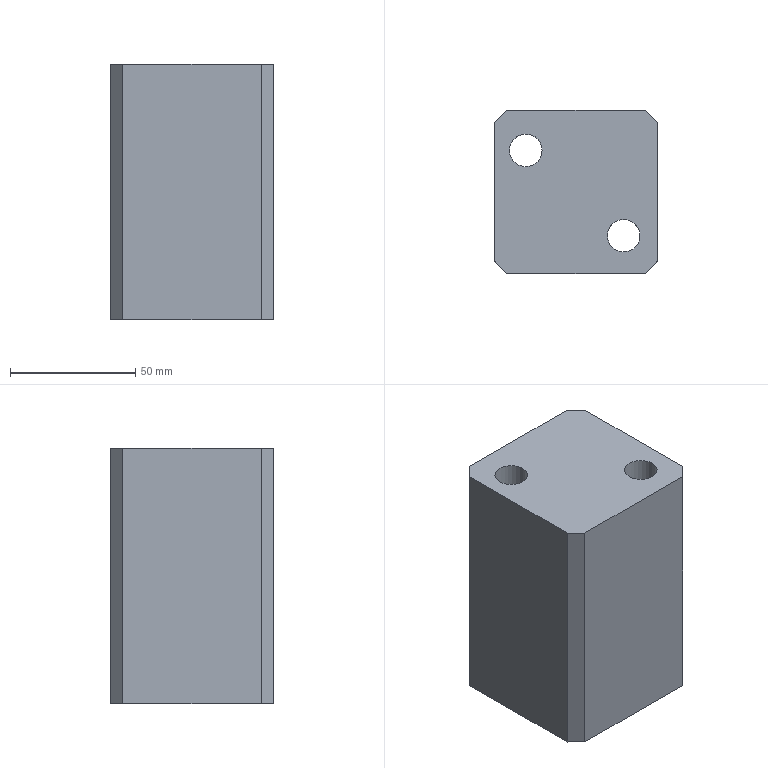Part | STEP file | gslz 2016.10.28-10_id2090_x_t | 1 solid | 20 faces | box 65 x 65 x 102 mm | volume 371101 mm3 | plane 12 | cylinder 6 | cone 2 | commonest cylinder face diameters 10.3 x2 13 x2 20 x2
STEP:
#1=CARTESIAN_POINT('',(0.,0.,0.));
#2=DIRECTION('',(0.,0.,1.));
#3=DIRECTION('',(1.,0.,0.));
#4=AXIS2_PLACEMENT_3D('',#1,#2,#3);
#5=CARTESIAN_POINT('',(-28.5,-279.,3.));
#6=VERTEX_POINT('',#5);
#7=CARTESIAN_POINT('',(-38.5,-279.,3.));
#8=DIRECTION('',(0.,0.,1.));
#9=DIRECTION('',(1.,0.,0.));
#10=AXIS2_PLACEMENT_3D('',#7,#8,#9);
#11=CIRCLE('',#10,10.);
#12=CARTESIAN_POINT('',(-339.5,-320.,3.));
#13=DIRECTION('',(0.,0.,1.));
#14=DIRECTION('',(0.,-1.,0.));
#15=AXIS2_PLACEMENT_3D('',#12,#13,#14);
#16=PLANE('',#15);
#17=CARTESIAN_POINT('',(-41.,301.));
#18=DIRECTION('',(0.,1.));
#19=AXIS2_PLACEMENT_2D('',#17,#18);
#20=CIRCLE('',#19,10.);
#21=(GEOMETRIC_REPRESENTATION_CONTEXT(2)PARAMETRIC_REPRESENTATION_CONTEXT()REPRESENTATION_CONTEXT('',''));
#22=DEFINITIONAL_REPRESENTATION('',(#20),#21);
#23=PCURVE('',#16,#22);
#24=CARTESIAN_POINT('',(-38.5,-279.,42.));
#25=DIRECTION('',(0.,0.,1.));
#26=DIRECTION('',(1.,0.,0.));
#27=AXIS2_PLACEMENT_3D('',#24,#25,#26);
#28=CYLINDRICAL_SURFACE('',#27,10.);
#29=CARTESIAN_POINT('',(0.,-39.));
#30=DIRECTION('',(1.,0.));
#31=VECTOR('',#30,1.);
#32=LINE('',#29,#31);
#33=(GEOMETRIC_REPRESENTATION_CONTEXT(2)PARAMETRIC_REPRESENTATION_CONTEXT()REPRESENTATION_CONTEXT('',''));
#34=DEFINITIONAL_REPRESENTATION('',(#32),#33);
#35=PCURVE('',#28,#34);
#36=SURFACE_CURVE('',#11,(#23,#35),.PCURVE_S1.);
#37=EDGE_CURVE('',#6,#6,#36,.T.);
#38=ORIENTED_EDGE('',*,*,#37,.T.);
#39=EDGE_LOOP('',(#38));
#40=FACE_BOUND('',#39,.T.);
#41=CARTESIAN_POINT('',(-51.,-267.929,3.));
#42=VERTEX_POINT('',#41);
#43=CARTESIAN_POINT('',(-51.,-323.071,3.));
#44=VERTEX_POINT('',#43);
#45=CARTESIAN_POINT('',(-51.,-320.,3.));
#46=DIRECTION('',(0.,-1.,0.));
#47=VECTOR('',#46,1.);
#48=LINE('',#45,#47);
#49=CARTESIAN_POINT('',(0.,288.5));
#50=DIRECTION('',(1.,0.));
#51=VECTOR('',#50,1.);
#52=LINE('',#49,#51);
#53=(GEOMETRIC_REPRESENTATION_CONTEXT(2)PARAMETRIC_REPRESENTATION_CONTEXT()REPRESENTATION_CONTEXT('',''));
#54=DEFINITIONAL_REPRESENTATION('',(#52),#53);
#55=PCURVE('',#16,#54);
#56=CARTESIAN_POINT('',(-51.,612.983,98.));
#57=DIRECTION('',(-1.,0.,0.));
#58=DIRECTION('',(0.,0.,1.));
#59=AXIS2_PLACEMENT_3D('',#56,#57,#58);
#60=PLANE('',#59);
#61=CARTESIAN_POINT('',(-95.,-932.983));
#62=DIRECTION('',(0.,-1.));
#63=VECTOR('',#62,1.);
#64=LINE('',#61,#63);
#65=(GEOMETRIC_REPRESENTATION_CONTEXT(2)PARAMETRIC_REPRESENTATION_CONTEXT()REPRESENTATION_CONTEXT('',''));
#66=DEFINITIONAL_REPRESENTATION('',(#64),#65);
#67=PCURVE('',#60,#66);
#68=SURFACE_CURVE('',#48,(#55,#67),.PCURVE_S1.);
#69=EDGE_CURVE('',#42,#44,#68,.T.);
#70=ORIENTED_EDGE('',*,*,#69,.F.);
#71=CARTESIAN_POINT('',(-46.071,-263.,3.));
#72=VERTEX_POINT('',#71);
#73=CARTESIAN_POINT('',(-47.536,-264.464,3.));
#74=DIRECTION('',(-0.7071,-0.7071,0.));
#75=VECTOR('',#74,1.);
#76=LINE('',#73,#75);
#77=CARTESIAN_POINT('',(-55.536,291.964));
#78=DIRECTION('',(0.7071,-0.7071));
#79=VECTOR('',#78,1.);
#80=LINE('',#77,#79);
#81=(GEOMETRIC_REPRESENTATION_CONTEXT(2)PARAMETRIC_REPRESENTATION_CONTEXT()REPRESENTATION_CONTEXT('',''));
#82=DEFINITIONAL_REPRESENTATION('',(#80),#81);
#83=PCURVE('',#16,#82);
#84=CARTESIAN_POINT('',(-47.536,-264.464,98.));
#85=DIRECTION('',(0.7071,-0.7071,0.));
#86=DIRECTION('',(0.,0.,1.));
#87=AXIS2_PLACEMENT_3D('',#84,#85,#86);
#88=PLANE('',#87);
#89=CARTESIAN_POINT('',(-95.,0.));
#90=DIRECTION('',(0.,1.));
#91=VECTOR('',#90,1.);
#92=LINE('',#89,#91);
#93=(GEOMETRIC_REPRESENTATION_CONTEXT(2)PARAMETRIC_REPRESENTATION_CONTEXT()REPRESENTATION_CONTEXT('',''));
#94=DEFINITIONAL_REPRESENTATION('',(#92),#93);
#95=PCURVE('',#88,#94);
#96=SURFACE_CURVE('',#76,(#83,#95),.PCURVE_S1.);
#97=EDGE_CURVE('',#72,#42,#96,.T.);
#98=ORIENTED_EDGE('',*,*,#97,.F.);
#99=CARTESIAN_POINT('',(9.071,-263.,3.));
#100=VERTEX_POINT('',#99);
#101=CARTESIAN_POINT('',(-339.5,-263.,3.));
#102=DIRECTION('',(-1.,0.,0.));
#103=VECTOR('',#102,1.);
#104=LINE('',#101,#103);
#105=CARTESIAN_POINT('',(-57.,0.));
#106=DIRECTION('',(0.,-1.));
#107=VECTOR('',#106,1.);
#108=LINE('',#105,#107);
#109=(GEOMETRIC_REPRESENTATION_CONTEXT(2)PARAMETRIC_REPRESENTATION_CONTEXT()REPRESENTATION_CONTEXT('',''));
#110=DEFINITIONAL_REPRESENTATION('',(#108),#109);
#111=PCURVE('',#16,#110);
#112=CARTESIAN_POINT('',(-677.884,-263.,98.));
#113=DIRECTION('',(0.,1.,0.));
#114=DIRECTION('',(1.,0.,0.));
#115=AXIS2_PLACEMENT_3D('',#112,#113,#114);
#116=PLANE('',#115);
#117=CARTESIAN_POINT('',(338.384,95.));
#118=DIRECTION('',(-1.,0.));
#119=VECTOR('',#118,1.);
#120=LINE('',#117,#119);
#121=(GEOMETRIC_REPRESENTATION_CONTEXT(2)PARAMETRIC_REPRESENTATION_CONTEXT()REPRESENTATION_CONTEXT('',''));
#122=DEFINITIONAL_REPRESENTATION('',(#120),#121);
#123=PCURVE('',#116,#122);
#124=SURFACE_CURVE('',#104,(#111,#123),.PCURVE_S1.);
#125=EDGE_CURVE('',#100,#72,#124,.T.);
#126=ORIENTED_EDGE('',*,*,#125,.F.);
#127=CARTESIAN_POINT('',(14.,-267.929,3.));
#128=VERTEX_POINT('',#127);
#129=CARTESIAN_POINT('',(12.536,-266.464,3.));
#130=DIRECTION('',(-0.7071,0.7071,0.));
#131=VECTOR('',#130,1.);
#132=LINE('',#129,#131);
#133=CARTESIAN_POINT('',(-53.536,352.036));
#134=DIRECTION('',(-0.7071,-0.7071));
#135=VECTOR('',#134,1.);
#136=LINE('',#133,#135);
#137=(GEOMETRIC_REPRESENTATION_CONTEXT(2)PARAMETRIC_REPRESENTATION_CONTEXT()REPRESENTATION_CONTEXT('',''));
#138=DEFINITIONAL_REPRESENTATION('',(#136),#137);
#139=PCURVE('',#16,#138);
#140=CARTESIAN_POINT('',(12.536,-266.464,98.));
#141=DIRECTION('',(-0.7071,-0.7071,0.));
#142=DIRECTION('',(0.,0.,1.));
#143=AXIS2_PLACEMENT_3D('',#140,#141,#142);
#144=PLANE('',#143);
#145=CARTESIAN_POINT('',(-95.,0.));
#146=DIRECTION('',(0.,1.));
#147=VECTOR('',#146,1.);
#148=LINE('',#145,#147);
#149=(GEOMETRIC_REPRESENTATION_CONTEXT(2)PARAMETRIC_REPRESENTATION_CONTEXT()REPRESENTATION_CONTEXT('',''));
#150=DEFINITIONAL_REPRESENTATION('',(#148),#149);
#151=PCURVE('',#144,#150);
#152=SURFACE_CURVE('',#132,(#139,#151),.PCURVE_S1.);
#153=EDGE_CURVE('',#128,#100,#152,.T.);
#154=ORIENTED_EDGE('',*,*,#153,.F.);
#155=CARTESIAN_POINT('',(14.,-323.071,3.));
#156=VERTEX_POINT('',#155);
#157=CARTESIAN_POINT('',(14.,-320.,3.));
#158=DIRECTION('',(0.,1.,0.));
#159=VECTOR('',#158,1.);
#160=LINE('',#157,#159);
#161=CARTESIAN_POINT('',(0.,353.5));
#162=DIRECTION('',(-1.,0.));
#163=VECTOR('',#162,1.);
#164=LINE('',#161,#163);
#165=(GEOMETRIC_REPRESENTATION_CONTEXT(2)PARAMETRIC_REPRESENTATION_CONTEXT()REPRESENTATION_CONTEXT('',''));
#166=DEFINITIONAL_REPRESENTATION('',(#164),#165);
#167=PCURVE('',#16,#166);
#168=CARTESIAN_POINT('',(14.,612.983,98.));
#169=DIRECTION('',(1.,0.,0.));
#170=DIRECTION('',(0.,0.,-1.));
#171=AXIS2_PLACEMENT_3D('',#168,#169,#170);
#172=PLANE('',#171);
#173=CARTESIAN_POINT('',(95.,-932.983));
#174=DIRECTION('',(0.,1.));
#175=VECTOR('',#174,1.);
#176=LINE('',#173,#175);
#177=(GEOMETRIC_REPRESENTATION_CONTEXT(2)PARAMETRIC_REPRESENTATION_CONTEXT()REPRESENTATION_CONTEXT('',''));
#178=DEFINITIONAL_REPRESENTATION('',(#176),#177);
#179=PCURVE('',#172,#178);
#180=SURFACE_CURVE('',#160,(#167,#179),.PCURVE_S1.);
#181=EDGE_CURVE('',#156,#128,#180,.T.);
#182=ORIENTED_EDGE('',*,*,#181,.F.);
#183=CARTESIAN_POINT('',(9.071,-328.,3.));
#184=VERTEX_POINT('',#183);
#185=CARTESIAN_POINT('',(12.536,-324.536,3.));
#186=DIRECTION('',(0.7071,0.7071,0.));
#187=VECTOR('',#186,1.);
#188=LINE('',#185,#187);
#189=CARTESIAN_POINT('',(4.536,352.036));
#190=DIRECTION('',(-0.7071,0.7071));
#191=VECTOR('',#190,1.);
#192=LINE('',#189,#191);
#193=(GEOMETRIC_REPRESENTATION_CONTEXT(2)PARAMETRIC_REPRESENTATION_CONTEXT()REPRESENTATION_CONTEXT('',''));
#194=DEFINITIONAL_REPRESENTATION('',(#192),#193);
#195=PCURVE('',#16,#194);
#196=CARTESIAN_POINT('',(12.536,-324.536,98.));
#197=DIRECTION('',(-0.7071,0.7071,0.));
#198=DIRECTION('',(0.,0.,-1.));
#199=AXIS2_PLACEMENT_3D('',#196,#197,#198);
#200=PLANE('',#199);
#201=CARTESIAN_POINT('',(95.,0.));
#202=DIRECTION('',(0.,-1.));
#203=VECTOR('',#202,1.);
#204=LINE('',#201,#203);
#205=(GEOMETRIC_REPRESENTATION_CONTEXT(2)PARAMETRIC_REPRESENTATION_CONTEXT()REPRESENTATION_CONTEXT('',''));
#206=DEFINITIONAL_REPRESENTATION('',(#204),#205);
#207=PCURVE('',#200,#206);
#208=SURFACE_CURVE('',#188,(#195,#207),.PCURVE_S1.);
#209=EDGE_CURVE('',#184,#156,#208,.T.);
#210=ORIENTED_EDGE('',*,*,#209,.F.);
#211=CARTESIAN_POINT('',(-46.071,-328.,3.));
#212=VERTEX_POINT('',#211);
#213=CARTESIAN_POINT('',(-339.5,-328.,3.));
#214=DIRECTION('',(1.,0.,0.));
#215=VECTOR('',#214,1.);
#216=LINE('',#213,#215);
#217=CARTESIAN_POINT('',(8.,0.));
#218=DIRECTION('',(0.,1.));
#219=VECTOR('',#218,1.);
#220=LINE('',#217,#219);
#221=(GEOMETRIC_REPRESENTATION_CONTEXT(2)PARAMETRIC_REPRESENTATION_CONTEXT()REPRESENTATION_CONTEXT('',''));
#222=DEFINITIONAL_REPRESENTATION('',(#220),#221);
#223=PCURVE('',#16,#222);
#224=CARTESIAN_POINT('',(-677.035,-328.,98.));
#225=DIRECTION('',(0.,-1.,0.));
#226=DIRECTION('',(-1.,0.,0.));
#227=AXIS2_PLACEMENT_3D('',#224,#225,#226);
#228=PLANE('',#227);
#229=CARTESIAN_POINT('',(-337.535,95.));
#230=DIRECTION('',(-1.,0.));
#231=VECTOR('',#230,1.);
#232=LINE('',#229,#231);
#233=(GEOMETRIC_REPRESENTATION_CONTEXT(2)PARAMETRIC_REPRESENTATION_CONTEXT()REPRESENTATION_CONTEXT('',''));
#234=DEFINITIONAL_REPRESENTATION('',(#232),#233);
#235=PCURVE('',#228,#234);
#236=SURFACE_CURVE('',#216,(#223,#235),.PCURVE_S1.);
#237=EDGE_CURVE('',#212,#184,#236,.T.);
#238=ORIENTED_EDGE('',*,*,#237,.F.);
#239=CARTESIAN_POINT('',(-47.536,-326.536,3.));
#240=DIRECTION('',(0.7071,-0.7071,0.));
#241=VECTOR('',#240,1.);
#242=LINE('',#239,#241);
#243=CARTESIAN_POINT('',(6.536,291.964));
#244=DIRECTION('',(0.7071,0.7071));
#245=VECTOR('',#244,1.);
#246=LINE('',#243,#245);
#247=(GEOMETRIC_REPRESENTATION_CONTEXT(2)PARAMETRIC_REPRESENTATION_CONTEXT()REPRESENTATION_CONTEXT('',''));
#248=DEFINITIONAL_REPRESENTATION('',(#246),#247);
#249=PCURVE('',#16,#248);
#250=CARTESIAN_POINT('',(-47.536,-326.536,98.));
#251=DIRECTION('',(0.7071,0.7071,0.));
#252=DIRECTION('',(0.,0.,-1.));
#253=AXIS2_PLACEMENT_3D('',#250,#251,#252);
#254=PLANE('',#253);
#255=CARTESIAN_POINT('',(95.,0.));
#256=DIRECTION('',(0.,-1.));
#257=VECTOR('',#256,1.);
#258=LINE('',#255,#257);
#259=(GEOMETRIC_REPRESENTATION_CONTEXT(2)PARAMETRIC_REPRESENTATION_CONTEXT()REPRESENTATION_CONTEXT('',''));
#260=DEFINITIONAL_REPRESENTATION('',(#258),#259);
#261=PCURVE('',#254,#260);
#262=SURFACE_CURVE('',#242,(#249,#261),.PCURVE_S1.);
#263=EDGE_CURVE('',#44,#212,#262,.T.);
#264=ORIENTED_EDGE('',*,*,#263,.F.);
#265=EDGE_LOOP('',(#70,#98,#126,#154,#182,#210,#238,#264));
#266=FACE_BOUND('',#265,.T.);
#267=CARTESIAN_POINT('',(10.5,-313.,3.));
#268=VERTEX_POINT('',#267);
#269=CARTESIAN_POINT('',(0.5,-313.,3.));
#270=DIRECTION('',(0.,0.,1.));
#271=DIRECTION('',(1.,0.,0.));
#272=AXIS2_PLACEMENT_3D('',#269,#270,#271);
#273=CIRCLE('',#272,10.);
#274=CARTESIAN_POINT('',(-7.,340.));
#275=DIRECTION('',(0.,1.));
#276=AXIS2_PLACEMENT_2D('',#274,#275);
#277=CIRCLE('',#276,10.);
#278=(GEOMETRIC_REPRESENTATION_CONTEXT(2)PARAMETRIC_REPRESENTATION_CONTEXT()REPRESENTATION_CONTEXT('',''));
#279=DEFINITIONAL_REPRESENTATION('',(#277),#278);
#280=PCURVE('',#16,#279);
#281=CARTESIAN_POINT('',(0.5,-313.,42.));
#282=DIRECTION('',(0.,0.,1.));
#283=DIRECTION('',(1.,0.,0.));
#284=AXIS2_PLACEMENT_3D('',#281,#282,#283);
#285=CYLINDRICAL_SURFACE('',#284,10.);
#286=CARTESIAN_POINT('',(0.,-39.));
#287=DIRECTION('',(1.,0.));
#288=VECTOR('',#287,1.);
#289=LINE('',#286,#288);
#290=(GEOMETRIC_REPRESENTATION_CONTEXT(2)PARAMETRIC_REPRESENTATION_CONTEXT()REPRESENTATION_CONTEXT('',''));
#291=DEFINITIONAL_REPRESENTATION('',(#289),#290);
#292=PCURVE('',#285,#291);
#293=SURFACE_CURVE('',#273,(#280,#292),.PCURVE_S1.);
#294=EDGE_CURVE('',#268,#268,#293,.T.);
#295=ORIENTED_EDGE('',*,*,#294,.T.);
#296=EDGE_LOOP('',(#295));
#297=FACE_BOUND('',#296,.T.);
#298=CARTESIAN_POINT('',(-33.35,-314.,3.));
#299=VERTEX_POINT('',#298);
#300=CARTESIAN_POINT('',(-38.5,-314.,3.));
#301=DIRECTION('',(0.,0.,-1.));
#302=DIRECTION('',(1.,0.,0.));
#303=AXIS2_PLACEMENT_3D('',#300,#301,#302);
#304=CIRCLE('',#303,5.15);
#305=CARTESIAN_POINT('',(-6.,306.15));
#306=CARTESIAN_POINT('',(2.92,306.15));
#307=CARTESIAN_POINT('',(-1.54,298.425));
#308=CARTESIAN_POINT('',(-6.,290.7));
#309=CARTESIAN_POINT('',(-10.46,298.425));
#310=CARTESIAN_POINT('',(-14.92,306.15));
#311=CARTESIAN_POINT('',(-6.,306.15));
#312=(BOUNDED_CURVE()B_SPLINE_CURVE(2,(#305,#306,#307,#308,#309,#310,#311),.UNSPECIFIED.,.T.,.F.)B_SPLINE_CURVE_WITH_KNOTS((1,2,2,2,2,1),(-2.094,0.,2.094,4.189,6.283,8.378),.UNSPECIFIED.)CURVE()GEOMETRIC_REPRESENTATION_ITEM()RATIONAL_B_SPLINE_CURVE((1.,0.5,1.,0.5,1.,0.5,1.))REPRESENTATION_ITEM(''));
#313=(GEOMETRIC_REPRESENTATION_CONTEXT(2)PARAMETRIC_REPRESENTATION_CONTEXT()REPRESENTATION_CONTEXT('',''));
#314=DEFINITIONAL_REPRESENTATION('',(#312),#313);
#315=PCURVE('',#16,#314);
#316=CARTESIAN_POINT('',(-38.5,-314.,-12.));
#317=DIRECTION('',(0.,0.,1.));
#318=DIRECTION('',(-1.,0.,0.));
#319=AXIS2_PLACEMENT_3D('',#316,#317,#318);
#320=CYLINDRICAL_SURFACE('',#319,5.15);
#321=CARTESIAN_POINT('',(9.425,15.));
#322=DIRECTION('',(-1.,0.));
#323=VECTOR('',#322,1.);
#324=LINE('',#321,#323);
#325=(GEOMETRIC_REPRESENTATION_CONTEXT(2)PARAMETRIC_REPRESENTATION_CONTEXT()REPRESENTATION_CONTEXT('',''));
#326=DEFINITIONAL_REPRESENTATION('',(#324),#325);
#327=PCURVE('',#320,#326);
#328=SURFACE_CURVE('',#304,(#315,#327),.PCURVE_S1.);
#329=EDGE_CURVE('',#299,#299,#328,.T.);
#330=ORIENTED_EDGE('',*,*,#329,.F.);
#331=EDGE_LOOP('',(#330));
#332=FACE_BOUND('',#331,.T.);
#333=CARTESIAN_POINT('',(5.65,-279.,3.));
#334=VERTEX_POINT('',#333);
#335=CARTESIAN_POINT('',(0.5,-279.,3.));
#336=DIRECTION('',(0.,0.,1.));
#337=DIRECTION('',(1.,0.,0.));
#338=AXIS2_PLACEMENT_3D('',#335,#336,#337);
#339=CIRCLE('',#338,5.15);
#340=CARTESIAN_POINT('',(-41.,340.));
#341=DIRECTION('',(0.,1.));
#342=AXIS2_PLACEMENT_2D('',#340,#341);
#343=CIRCLE('',#342,5.15);
#344=(GEOMETRIC_REPRESENTATION_CONTEXT(2)PARAMETRIC_REPRESENTATION_CONTEXT()REPRESENTATION_CONTEXT('',''));
#345=DEFINITIONAL_REPRESENTATION('',(#343),#344);
#346=PCURVE('',#16,#345);
#347=CARTESIAN_POINT('',(0.5,-279.,-12.));
#348=DIRECTION('',(0.,0.,1.));
#349=DIRECTION('',(-1.,0.,0.));
#350=AXIS2_PLACEMENT_3D('',#347,#348,#349);
#351=CYLINDRICAL_SURFACE('',#350,5.15);
#352=CARTESIAN_POINT('',(3.142,15.));
#353=DIRECTION('',(1.,0.));
#354=VECTOR('',#353,1.);
#355=LINE('',#352,#354);
#356=(GEOMETRIC_REPRESENTATION_CONTEXT(2)PARAMETRIC_REPRESENTATION_CONTEXT()REPRESENTATION_CONTEXT('',''));
#357=DEFINITIONAL_REPRESENTATION('',(#355),#356);
#358=PCURVE('',#351,#357);
#359=SURFACE_CURVE('',#339,(#346,#358),.PCURVE_S1.);
#360=EDGE_CURVE('',#334,#334,#359,.T.);
#361=ORIENTED_EDGE('',*,*,#360,.T.);
#362=EDGE_LOOP('',(#361));
#363=FACE_BOUND('',#362,.T.);
#364=ADVANCED_FACE('',(#40,#266,#297,#332,#363),#16,.F.);
#365=CARTESIAN_POINT('',(-33.35,-314.,23.));
#366=VERTEX_POINT('',#365);
#367=CARTESIAN_POINT('',(-38.5,-314.,23.));
#368=DIRECTION('',(0.,0.,1.));
#369=DIRECTION('',(1.,0.,0.));
#370=AXIS2_PLACEMENT_3D('',#367,#368,#369);
#371=CIRCLE('',#370,5.15);
#372=CARTESIAN_POINT('',(3.142,35.));
#373=DIRECTION('',(1.,0.));
#374=VECTOR('',#373,1.);
#375=LINE('',#372,#374);
#376=(GEOMETRIC_REPRESENTATION_CONTEXT(2)PARAMETRIC_REPRESENTATION_CONTEXT()REPRESENTATION_CONTEXT('',''));
#377=DEFINITIONAL_REPRESENTATION('',(#375),#376);
#378=PCURVE('',#320,#377);
#379=CARTESIAN_POINT('',(-38.5,-314.,23.));
#380=DIRECTION('',(0.,0.,-1.));
#381=DIRECTION('',(1.,0.,0.));
#382=AXIS2_PLACEMENT_3D('',#379,#380,#381);
#383=CONICAL_SURFACE('',#382,5.15,1.03);
#384=CARTESIAN_POINT('',(6.283,0.));
#385=DIRECTION('',(-1.,0.));
#386=VECTOR('',#385,1.);
#387=LINE('',#384,#386);
#388=(GEOMETRIC_REPRESENTATION_CONTEXT(2)PARAMETRIC_REPRESENTATION_CONTEXT()REPRESENTATION_CONTEXT('',''));
#389=DEFINITIONAL_REPRESENTATION('',(#387),#388);
#390=PCURVE('',#383,#389);
#391=SURFACE_CURVE('',#371,(#378,#390),.PCURVE_S1.);
#392=EDGE_CURVE('',#366,#366,#391,.T.);
#393=ORIENTED_EDGE('',*,*,#392,.F.);
#394=CARTESIAN_POINT('',(-33.35,-314.,3.));
#395=CARTESIAN_POINT('',(-33.35,-314.,23.));
#396=B_SPLINE_CURVE_WITH_KNOTS('',1,(#394,#395),.UNSPECIFIED.,.F.,.F.,(2,2),(15.,35.),.PIECEWISE_BEZIER_KNOTS.);
#397=CARTESIAN_POINT('',(3.142,0.));
#398=DIRECTION('',(0.,1.));
#399=VECTOR('',#398,1.);
#400=LINE('',#397,#399);
#401=(GEOMETRIC_REPRESENTATION_CONTEXT(2)PARAMETRIC_REPRESENTATION_CONTEXT()REPRESENTATION_CONTEXT('',''));
#402=DEFINITIONAL_REPRESENTATION('',(#400),#401);
#403=PCURVE('',#320,#402);
#404=CARTESIAN_POINT('',(9.425,0.));
#405=DIRECTION('',(0.,1.));
#406=VECTOR('',#405,1.);
#407=LINE('',#404,#406);
#408=(GEOMETRIC_REPRESENTATION_CONTEXT(2)PARAMETRIC_REPRESENTATION_CONTEXT()REPRESENTATION_CONTEXT('',''));
#409=DEFINITIONAL_REPRESENTATION('',(#407),#408);
#410=PCURVE('',#320,#409);
#411=SEAM_CURVE('',#396,(#403,#410),.PCURVE_S1.);
#412=EDGE_CURVE('',#299,#366,#411,.T.);
#413=ORIENTED_EDGE('',*,*,#412,.F.);
#414=ORIENTED_EDGE('',*,*,#329,.F.);
#415=ORIENTED_EDGE('',*,*,#412,.T.);
#416=EDGE_LOOP('',(#393,#413,#414,#415));
#417=FACE_BOUND('',#416,.F.);
#418=ADVANCED_FACE('',(#417),#320,.F.);
#419=CARTESIAN_POINT('',(7.,-313.,70.));
#420=VERTEX_POINT('',#419);
#421=CARTESIAN_POINT('',(0.5,-313.,70.));
#422=DIRECTION('',(0.,0.,1.));
#423=DIRECTION('',(1.,0.,0.));
#424=AXIS2_PLACEMENT_3D('',#421,#422,#423);
#425=CIRCLE('',#424,6.5);
#426=CARTESIAN_POINT('',(0.5,-313.,70.));
#427=DIRECTION('',(0.,0.,1.));
#428=DIRECTION('',(1.,0.,0.));
#429=AXIS2_PLACEMENT_3D('',#426,#427,#428);
#430=PLANE('',#429);
#431=CARTESIAN_POINT('',(0.,0.));
#432=DIRECTION('',(1.,0.));
#433=AXIS2_PLACEMENT_2D('',#431,#432);
#434=CIRCLE('',#433,6.5);
#435=(GEOMETRIC_REPRESENTATION_CONTEXT(2)PARAMETRIC_REPRESENTATION_CONTEXT()REPRESENTATION_CONTEXT('',''));
#436=DEFINITIONAL_REPRESENTATION('',(#434),#435);
#437=PCURVE('',#430,#436);
#438=CARTESIAN_POINT('',(0.5,-313.,87.));
#439=DIRECTION('',(0.,0.,1.));
#440=DIRECTION('',(1.,0.,0.));
#441=AXIS2_PLACEMENT_3D('',#438,#439,#440);
#442=CYLINDRICAL_SURFACE('',#441,6.5);
#443=CARTESIAN_POINT('',(0.,-17.));
#444=DIRECTION('',(1.,0.));
#445=VECTOR('',#444,1.);
#446=LINE('',#443,#445);
#447=(GEOMETRIC_REPRESENTATION_CONTEXT(2)PARAMETRIC_REPRESENTATION_CONTEXT()REPRESENTATION_CONTEXT('',''));
#448=DEFINITIONAL_REPRESENTATION('',(#446),#447);
#449=PCURVE('',#442,#448);
#450=SURFACE_CURVE('',#425,(#437,#449),.PCURVE_S1.);
#451=EDGE_CURVE('',#420,#420,#450,.T.);
#452=ORIENTED_EDGE('',*,*,#451,.T.);
#453=EDGE_LOOP('',(#452));
#454=FACE_BOUND('',#453,.T.);
#455=CARTESIAN_POINT('',(10.5,-313.,70.));
#456=VERTEX_POINT('',#455);
#457=CARTESIAN_POINT('',(0.5,-313.,70.));
#458=DIRECTION('',(0.,0.,1.));
#459=DIRECTION('',(1.,0.,0.));
#460=AXIS2_PLACEMENT_3D('',#457,#458,#459);
#461=CIRCLE('',#460,10.);
#462=CARTESIAN_POINT('',(0.,0.));
#463=DIRECTION('',(1.,0.));
#464=AXIS2_PLACEMENT_2D('',#462,#463);
#465=CIRCLE('',#464,10.);
#466=(GEOMETRIC_REPRESENTATION_CONTEXT(2)PARAMETRIC_REPRESENTATION_CONTEXT()REPRESENTATION_CONTEXT('',''));
#467=DEFINITIONAL_REPRESENTATION('',(#465),#466);
#468=PCURVE('',#430,#467);
#469=CARTESIAN_POINT('',(0.,28.));
#470=DIRECTION('',(1.,0.));
#471=VECTOR('',#470,1.);
#472=LINE('',#469,#471);
#473=(GEOMETRIC_REPRESENTATION_CONTEXT(2)PARAMETRIC_REPRESENTATION_CONTEXT()REPRESENTATION_CONTEXT('',''));
#474=DEFINITIONAL_REPRESENTATION('',(#472),#473);
#475=PCURVE('',#285,#474);
#476=SURFACE_CURVE('',#461,(#468,#475),.PCURVE_S1.);
#477=EDGE_CURVE('',#456,#456,#476,.T.);
#478=ORIENTED_EDGE('',*,*,#477,.F.);
#479=EDGE_LOOP('',(#478));
#480=FACE_BOUND('',#479,.T.);
#481=ADVANCED_FACE('',(#454,#480),#430,.F.);
#482=CARTESIAN_POINT('',(-32.,-279.,70.));
#483=VERTEX_POINT('',#482);
#484=CARTESIAN_POINT('',(-38.5,-279.,70.));
#485=DIRECTION('',(0.,0.,1.));
#486=DIRECTION('',(1.,0.,0.));
#487=AXIS2_PLACEMENT_3D('',#484,#485,#486);
#488=CIRCLE('',#487,6.5);
#489=CARTESIAN_POINT('',(-38.5,-279.,70.));
#490=DIRECTION('',(0.,0.,1.));
#491=DIRECTION('',(1.,0.,0.));
#492=AXIS2_PLACEMENT_3D('',#489,#490,#491);
#493=PLANE('',#492);
#494=CARTESIAN_POINT('',(0.,0.));
#495=DIRECTION('',(1.,0.));
#496=AXIS2_PLACEMENT_2D('',#494,#495);
#497=CIRCLE('',#496,6.5);
#498=(GEOMETRIC_REPRESENTATION_CONTEXT(2)PARAMETRIC_REPRESENTATION_CONTEXT()REPRESENTATION_CONTEXT('',''));
#499=DEFINITIONAL_REPRESENTATION('',(#497),#498);
#500=PCURVE('',#493,#499);
#501=CARTESIAN_POINT('',(-38.5,-279.,87.));
#502=DIRECTION('',(0.,0.,1.));
#503=DIRECTION('',(1.,0.,0.));
#504=AXIS2_PLACEMENT_3D('',#501,#502,#503);
#505=CYLINDRICAL_SURFACE('',#504,6.5);
#506=CARTESIAN_POINT('',(0.,-17.));
#507=DIRECTION('',(1.,0.));
#508=VECTOR('',#507,1.);
#509=LINE('',#506,#508);
#510=(GEOMETRIC_REPRESENTATION_CONTEXT(2)PARAMETRIC_REPRESENTATION_CONTEXT()REPRESENTATION_CONTEXT('',''));
#511=DEFINITIONAL_REPRESENTATION('',(#509),#510);
#512=PCURVE('',#505,#511);
#513=SURFACE_CURVE('',#488,(#500,#512),.PCURVE_S1.);
#514=EDGE_CURVE('',#483,#483,#513,.T.);
#515=ORIENTED_EDGE('',*,*,#514,.T.);
#516=EDGE_LOOP('',(#515));
#517=FACE_BOUND('',#516,.T.);
#518=CARTESIAN_POINT('',(-28.5,-279.,70.));
#519=VERTEX_POINT('',#518);
#520=CARTESIAN_POINT('',(-38.5,-279.,70.));
#521=DIRECTION('',(0.,0.,1.));
#522=DIRECTION('',(1.,0.,0.));
#523=AXIS2_PLACEMENT_3D('',#520,#521,#522);
#524=CIRCLE('',#523,10.);
#525=CARTESIAN_POINT('',(0.,0.));
#526=DIRECTION('',(1.,0.));
#527=AXIS2_PLACEMENT_2D('',#525,#526);
#528=CIRCLE('',#527,10.);
#529=(GEOMETRIC_REPRESENTATION_CONTEXT(2)PARAMETRIC_REPRESENTATION_CONTEXT()REPRESENTATION_CONTEXT('',''));
#530=DEFINITIONAL_REPRESENTATION('',(#528),#529);
#531=PCURVE('',#493,#530);
#532=CARTESIAN_POINT('',(0.,28.));
#533=DIRECTION('',(1.,0.));
#534=VECTOR('',#533,1.);
#535=LINE('',#532,#534);
#536=(GEOMETRIC_REPRESENTATION_CONTEXT(2)PARAMETRIC_REPRESENTATION_CONTEXT()REPRESENTATION_CONTEXT('',''));
#537=DEFINITIONAL_REPRESENTATION('',(#535),#536);
#538=PCURVE('',#28,#537);
#539=SURFACE_CURVE('',#524,(#531,#538),.PCURVE_S1.);
#540=EDGE_CURVE('',#519,#519,#539,.T.);
#541=ORIENTED_EDGE('',*,*,#540,.F.);
#542=EDGE_LOOP('',(#541));
#543=FACE_BOUND('',#542,.T.);
#544=ADVANCED_FACE('',(#517,#543),#493,.F.);
#545=ORIENTED_EDGE('',*,*,#294,.T.);
#546=CARTESIAN_POINT('',(10.5,-313.,3.));
#547=CARTESIAN_POINT('',(10.5,-313.,70.));
#548=B_SPLINE_CURVE_WITH_KNOTS('',1,(#546,#547),.UNSPECIFIED.,.F.,.F.,(2,2),(-39.,28.),.PIECEWISE_BEZIER_KNOTS.);
#549=CARTESIAN_POINT('',(6.283,0.));
#550=DIRECTION('',(0.,1.));
#551=VECTOR('',#550,1.);
#552=LINE('',#549,#551);
#553=(GEOMETRIC_REPRESENTATION_CONTEXT(2)PARAMETRIC_REPRESENTATION_CONTEXT()REPRESENTATION_CONTEXT('',''));
#554=DEFINITIONAL_REPRESENTATION('',(#552),#553);
#555=PCURVE('',#285,#554);
#556=CARTESIAN_POINT('',(0.,0.));
#557=DIRECTION('',(0.,1.));
#558=VECTOR('',#557,1.);
#559=LINE('',#556,#558);
#560=(GEOMETRIC_REPRESENTATION_CONTEXT(2)PARAMETRIC_REPRESENTATION_CONTEXT()REPRESENTATION_CONTEXT('',''));
#561=DEFINITIONAL_REPRESENTATION('',(#559),#560);
#562=PCURVE('',#285,#561);
#563=SEAM_CURVE('',#548,(#555,#562),.PCURVE_S1.);
#564=EDGE_CURVE('',#268,#456,#563,.T.);
#565=ORIENTED_EDGE('',*,*,#564,.T.);
#566=ORIENTED_EDGE('',*,*,#477,.F.);
#567=ORIENTED_EDGE('',*,*,#564,.F.);
#568=EDGE_LOOP('',(#545,#565,#566,#567));
#569=FACE_BOUND('',#568,.F.);
#570=ADVANCED_FACE('',(#569),#285,.F.);
#571=ORIENTED_EDGE('',*,*,#237,.T.);
#572=CARTESIAN_POINT('',(9.071,-328.,105.));
#573=VERTEX_POINT('',#572);
#574=CARTESIAN_POINT('',(9.071,-328.,98.));
#575=DIRECTION('',(0.,0.,-1.));
#576=VECTOR('',#575,1.);
#577=LINE('',#574,#576);
#578=CARTESIAN_POINT('',(-686.106,0.));
#579=DIRECTION('',(0.,1.));
#580=VECTOR('',#579,1.);
#581=LINE('',#578,#580);
#582=(GEOMETRIC_REPRESENTATION_CONTEXT(2)PARAMETRIC_REPRESENTATION_CONTEXT()REPRESENTATION_CONTEXT('',''));
#583=DEFINITIONAL_REPRESENTATION('',(#581),#582);
#584=PCURVE('',#228,#583);
#585=CARTESIAN_POINT('',(0.,4.899));
#586=DIRECTION('',(1.,0.));
#587=VECTOR('',#586,1.);
#588=LINE('',#585,#587);
#589=(GEOMETRIC_REPRESENTATION_CONTEXT(2)PARAMETRIC_REPRESENTATION_CONTEXT()REPRESENTATION_CONTEXT('',''));
#590=DEFINITIONAL_REPRESENTATION('',(#588),#589);
#591=PCURVE('',#200,#590);
#592=SURFACE_CURVE('',#577,(#584,#591),.PCURVE_S1.);
#593=EDGE_CURVE('',#573,#184,#592,.T.);
#594=ORIENTED_EDGE('',*,*,#593,.F.);
#595=CARTESIAN_POINT('',(-46.071,-328.,105.));
#596=VERTEX_POINT('',#595);
#597=CARTESIAN_POINT('',(46.5,-328.,105.));
#598=DIRECTION('',(1.,0.,0.));
#599=VECTOR('',#598,1.);
#600=LINE('',#597,#599);
#601=CARTESIAN_POINT('',(-723.535,-7.));
#602=DIRECTION('',(-1.,0.));
#603=VECTOR('',#602,1.);
#604=LINE('',#601,#603);
#605=(GEOMETRIC_REPRESENTATION_CONTEXT(2)PARAMETRIC_REPRESENTATION_CONTEXT()REPRESENTATION_CONTEXT('',''));
#606=DEFINITIONAL_REPRESENTATION('',(#604),#605);
#607=PCURVE('',#228,#606);
#608=CARTESIAN_POINT('',(46.5,87.,105.));
#609=DIRECTION('',(0.,0.,1.));
#610=DIRECTION('',(-1.,0.,0.));
#611=AXIS2_PLACEMENT_3D('',#608,#609,#610);
#612=PLANE('',#611);
#613=CARTESIAN_POINT('',(0.,415.));
#614=DIRECTION('',(-1.,0.));
#615=VECTOR('',#614,1.);
#616=LINE('',#613,#615);
#617=(GEOMETRIC_REPRESENTATION_CONTEXT(2)PARAMETRIC_REPRESENTATION_CONTEXT()REPRESENTATION_CONTEXT('',''));
#618=DEFINITIONAL_REPRESENTATION('',(#616),#617);
#619=PCURVE('',#612,#618);
#620=SURFACE_CURVE('',#600,(#607,#619),.PCURVE_S1.);
#621=EDGE_CURVE('',#596,#573,#620,.T.);
#622=ORIENTED_EDGE('',*,*,#621,.F.);
#623=CARTESIAN_POINT('',(-46.071,-328.,98.));
#624=DIRECTION('',(0.,0.,1.));
#625=VECTOR('',#624,1.);
#626=LINE('',#623,#625);
#627=CARTESIAN_POINT('',(-630.964,0.));
#628=DIRECTION('',(0.,-1.));
#629=VECTOR('',#628,1.);
#630=LINE('',#627,#629);
#631=(GEOMETRIC_REPRESENTATION_CONTEXT(2)PARAMETRIC_REPRESENTATION_CONTEXT()REPRESENTATION_CONTEXT('',''));
#632=DEFINITIONAL_REPRESENTATION('',(#630),#631);
#633=PCURVE('',#228,#632);
#634=CARTESIAN_POINT('',(0.,-2.071));
#635=DIRECTION('',(-1.,0.));
#636=VECTOR('',#635,1.);
#637=LINE('',#634,#636);
#638=(GEOMETRIC_REPRESENTATION_CONTEXT(2)PARAMETRIC_REPRESENTATION_CONTEXT()REPRESENTATION_CONTEXT('',''));
#639=DEFINITIONAL_REPRESENTATION('',(#637),#638);
#640=PCURVE('',#254,#639);
#641=SURFACE_CURVE('',#626,(#633,#640),.PCURVE_S1.);
#642=EDGE_CURVE('',#212,#596,#641,.T.);
#643=ORIENTED_EDGE('',*,*,#642,.F.);
#644=EDGE_LOOP('',(#571,#594,#622,#643));
#645=FACE_BOUND('',#644,.T.);
#646=ADVANCED_FACE('',(#645),#228,.T.);
#647=CARTESIAN_POINT('',(-51.,-267.929,105.));
#648=VERTEX_POINT('',#647);
#649=CARTESIAN_POINT('',(-51.,-323.071,105.));
#650=VERTEX_POINT('',#649);
#651=CARTESIAN_POINT('',(-51.,87.,105.));
#652=DIRECTION('',(0.,-1.,0.));
#653=VECTOR('',#652,1.);
#654=LINE('',#651,#653);
#655=CARTESIAN_POINT('',(7.,-525.983));
#656=DIRECTION('',(0.,-1.));
#657=VECTOR('',#656,1.);
#658=LINE('',#655,#657);
#659=(GEOMETRIC_REPRESENTATION_CONTEXT(2)PARAMETRIC_REPRESENTATION_CONTEXT()REPRESENTATION_CONTEXT('',''));
#660=DEFINITIONAL_REPRESENTATION('',(#658),#659);
#661=PCURVE('',#60,#660);
#662=CARTESIAN_POINT('',(97.5,0.));
#663=DIRECTION('',(0.,1.));
#664=VECTOR('',#663,1.);
#665=LINE('',#662,#664);
#666=(GEOMETRIC_REPRESENTATION_CONTEXT(2)PARAMETRIC_REPRESENTATION_CONTEXT()REPRESENTATION_CONTEXT('',''));
#667=DEFINITIONAL_REPRESENTATION('',(#665),#666);
#668=PCURVE('',#612,#667);
#669=SURFACE_CURVE('',#654,(#661,#668),.PCURVE_S1.);
#670=EDGE_CURVE('',#648,#650,#669,.T.);
#671=ORIENTED_EDGE('',*,*,#670,.F.);
#672=CARTESIAN_POINT('',(-51.,-267.929,98.));
#673=DIRECTION('',(0.,0.,1.));
#674=VECTOR('',#673,1.);
#675=LINE('',#672,#674);
#676=CARTESIAN_POINT('',(0.,-880.911));
#677=DIRECTION('',(1.,0.));
#678=VECTOR('',#677,1.);
#679=LINE('',#676,#678);
#680=(GEOMETRIC_REPRESENTATION_CONTEXT(2)PARAMETRIC_REPRESENTATION_CONTEXT()REPRESENTATION_CONTEXT('',''));
#681=DEFINITIONAL_REPRESENTATION('',(#679),#680);
#682=PCURVE('',#60,#681);
#683=CARTESIAN_POINT('',(0.,4.899));
#684=DIRECTION('',(1.,0.));
#685=VECTOR('',#684,1.);
#686=LINE('',#683,#685);
#687=(GEOMETRIC_REPRESENTATION_CONTEXT(2)PARAMETRIC_REPRESENTATION_CONTEXT()REPRESENTATION_CONTEXT('',''));
#688=DEFINITIONAL_REPRESENTATION('',(#686),#687);
#689=PCURVE('',#88,#688);
#690=SURFACE_CURVE('',#675,(#682,#689),.PCURVE_S1.);
#691=EDGE_CURVE('',#42,#648,#690,.T.);
#692=ORIENTED_EDGE('',*,*,#691,.F.);
#693=ORIENTED_EDGE('',*,*,#69,.T.);
#694=CARTESIAN_POINT('',(-51.,-323.071,98.));
#695=DIRECTION('',(0.,0.,-1.));
#696=VECTOR('',#695,1.);
#697=LINE('',#694,#696);
#698=CARTESIAN_POINT('',(0.,-936.054));
#699=DIRECTION('',(-1.,0.));
#700=VECTOR('',#699,1.);
#701=LINE('',#698,#700);
#702=(GEOMETRIC_REPRESENTATION_CONTEXT(2)PARAMETRIC_REPRESENTATION_CONTEXT()REPRESENTATION_CONTEXT('',''));
#703=DEFINITIONAL_REPRESENTATION('',(#701),#702);
#704=PCURVE('',#60,#703);
#705=CARTESIAN_POINT('',(0.,4.899));
#706=DIRECTION('',(1.,0.));
#707=VECTOR('',#706,1.);
#708=LINE('',#705,#707);
#709=(GEOMETRIC_REPRESENTATION_CONTEXT(2)PARAMETRIC_REPRESENTATION_CONTEXT()REPRESENTATION_CONTEXT('',''));
#710=DEFINITIONAL_REPRESENTATION('',(#708),#709);
#711=PCURVE('',#254,#710);
#712=SURFACE_CURVE('',#697,(#704,#711),.PCURVE_S1.);
#713=EDGE_CURVE('',#650,#44,#712,.T.);
#714=ORIENTED_EDGE('',*,*,#713,.F.);
#715=EDGE_LOOP('',(#671,#692,#693,#714));
#716=FACE_BOUND('',#715,.T.);
#717=ADVANCED_FACE('',(#716),#60,.T.);
#718=CARTESIAN_POINT('',(9.071,-263.,105.));
#719=VERTEX_POINT('',#718);
#720=CARTESIAN_POINT('',(-46.071,-263.,105.));
#721=VERTEX_POINT('',#720);
#722=CARTESIAN_POINT('',(46.5,-263.,105.));
#723=DIRECTION('',(-1.,0.,0.));
#724=VECTOR('',#723,1.);
#725=LINE('',#722,#724);
#726=CARTESIAN_POINT('',(724.384,-7.));
#727=DIRECTION('',(-1.,0.));
#728=VECTOR('',#727,1.);
#729=LINE('',#726,#728);
#730=(GEOMETRIC_REPRESENTATION_CONTEXT(2)PARAMETRIC_REPRESENTATION_CONTEXT()REPRESENTATION_CONTEXT('',''));
#731=DEFINITIONAL_REPRESENTATION('',(#729),#730);
#732=PCURVE('',#116,#731);
#733=CARTESIAN_POINT('',(0.,350.));
#734=DIRECTION('',(1.,0.));
#735=VECTOR('',#734,1.);
#736=LINE('',#733,#735);
#737=(GEOMETRIC_REPRESENTATION_CONTEXT(2)PARAMETRIC_REPRESENTATION_CONTEXT()REPRESENTATION_CONTEXT('',''));
#738=DEFINITIONAL_REPRESENTATION('',(#736),#737);
#739=PCURVE('',#612,#738);
#740=SURFACE_CURVE('',#725,(#732,#739),.PCURVE_S1.);
#741=EDGE_CURVE('',#719,#721,#740,.T.);
#742=ORIENTED_EDGE('',*,*,#741,.F.);
#743=CARTESIAN_POINT('',(9.071,-263.,98.));
#744=DIRECTION('',(0.,0.,1.));
#745=VECTOR('',#744,1.);
#746=LINE('',#743,#745);
#747=CARTESIAN_POINT('',(686.955,0.));
#748=DIRECTION('',(0.,-1.));
#749=VECTOR('',#748,1.);
#750=LINE('',#747,#749);
#751=(GEOMETRIC_REPRESENTATION_CONTEXT(2)PARAMETRIC_REPRESENTATION_CONTEXT()REPRESENTATION_CONTEXT('',''));
#752=DEFINITIONAL_REPRESENTATION('',(#750),#751);
#753=PCURVE('',#116,#752);
#754=CARTESIAN_POINT('',(0.,4.899));
#755=DIRECTION('',(1.,0.));
#756=VECTOR('',#755,1.);
#757=LINE('',#754,#756);
#758=(GEOMETRIC_REPRESENTATION_CONTEXT(2)PARAMETRIC_REPRESENTATION_CONTEXT()REPRESENTATION_CONTEXT('',''));
#759=DEFINITIONAL_REPRESENTATION('',(#757),#758);
#760=PCURVE('',#144,#759);
#761=SURFACE_CURVE('',#746,(#753,#760),.PCURVE_S1.);
#762=EDGE_CURVE('',#100,#719,#761,.T.);
#763=ORIENTED_EDGE('',*,*,#762,.F.);
#764=ORIENTED_EDGE('',*,*,#125,.T.);
#765=CARTESIAN_POINT('',(-46.071,-263.,98.));
#766=DIRECTION('',(0.,0.,-1.));
#767=VECTOR('',#766,1.);
#768=LINE('',#765,#767);
#769=CARTESIAN_POINT('',(631.812,0.));
#770=DIRECTION('',(0.,1.));
#771=VECTOR('',#770,1.);
#772=LINE('',#769,#771);
#773=(GEOMETRIC_REPRESENTATION_CONTEXT(2)PARAMETRIC_REPRESENTATION_CONTEXT()REPRESENTATION_CONTEXT('',''));
#774=DEFINITIONAL_REPRESENTATION('',(#772),#773);
#775=PCURVE('',#116,#774);
#776=CARTESIAN_POINT('',(0.,-2.071));
#777=DIRECTION('',(-1.,0.));
#778=VECTOR('',#777,1.);
#779=LINE('',#776,#778);
#780=(GEOMETRIC_REPRESENTATION_CONTEXT(2)PARAMETRIC_REPRESENTATION_CONTEXT()REPRESENTATION_CONTEXT('',''));
#781=DEFINITIONAL_REPRESENTATION('',(#779),#780);
#782=PCURVE('',#88,#781);
#783=SURFACE_CURVE('',#768,(#775,#782),.PCURVE_S1.);
#784=EDGE_CURVE('',#721,#72,#783,.T.);
#785=ORIENTED_EDGE('',*,*,#784,.F.);
#786=EDGE_LOOP('',(#742,#763,#764,#785));
#787=FACE_BOUND('',#786,.T.);
#788=ADVANCED_FACE('',(#787),#116,.T.);
#789=CARTESIAN_POINT('',(14.,-323.071,105.));
#790=VERTEX_POINT('',#789);
#791=CARTESIAN_POINT('',(14.,-267.929,105.));
#792=VERTEX_POINT('',#791);
#793=CARTESIAN_POINT('',(14.,87.,105.));
#794=DIRECTION('',(0.,1.,0.));
#795=VECTOR('',#794,1.);
#796=LINE('',#793,#795);
#797=CARTESIAN_POINT('',(-7.,-525.983));
#798=DIRECTION('',(0.,1.));
#799=VECTOR('',#798,1.);
#800=LINE('',#797,#799);
#801=(GEOMETRIC_REPRESENTATION_CONTEXT(2)PARAMETRIC_REPRESENTATION_CONTEXT()REPRESENTATION_CONTEXT('',''));
#802=DEFINITIONAL_REPRESENTATION('',(#800),#801);
#803=PCURVE('',#172,#802);
#804=CARTESIAN_POINT('',(32.5,0.));
#805=DIRECTION('',(0.,-1.));
#806=VECTOR('',#805,1.);
#807=LINE('',#804,#806);
#808=(GEOMETRIC_REPRESENTATION_CONTEXT(2)PARAMETRIC_REPRESENTATION_CONTEXT()REPRESENTATION_CONTEXT('',''));
#809=DEFINITIONAL_REPRESENTATION('',(#807),#808);
#810=PCURVE('',#612,#809);
#811=SURFACE_CURVE('',#796,(#803,#810),.PCURVE_S1.);
#812=EDGE_CURVE('',#790,#792,#811,.T.);
#813=ORIENTED_EDGE('',*,*,#812,.F.);
#814=CARTESIAN_POINT('',(14.,-323.071,98.));
#815=DIRECTION('',(0.,0.,1.));
#816=VECTOR('',#815,1.);
#817=LINE('',#814,#816);
#818=CARTESIAN_POINT('',(0.,-936.054));
#819=DIRECTION('',(-1.,0.));
#820=VECTOR('',#819,1.);
#821=LINE('',#818,#820);
#822=(GEOMETRIC_REPRESENTATION_CONTEXT(2)PARAMETRIC_REPRESENTATION_CONTEXT()REPRESENTATION_CONTEXT('',''));
#823=DEFINITIONAL_REPRESENTATION('',(#821),#822);
#824=PCURVE('',#172,#823);
#825=CARTESIAN_POINT('',(0.,-2.071));
#826=DIRECTION('',(-1.,0.));
#827=VECTOR('',#826,1.);
#828=LINE('',#825,#827);
#829=(GEOMETRIC_REPRESENTATION_CONTEXT(2)PARAMETRIC_REPRESENTATION_CONTEXT()REPRESENTATION_CONTEXT('',''));
#830=DEFINITIONAL_REPRESENTATION('',(#828),#829);
#831=PCURVE('',#200,#830);
#832=SURFACE_CURVE('',#817,(#824,#831),.PCURVE_S1.);
#833=EDGE_CURVE('',#156,#790,#832,.T.);
#834=ORIENTED_EDGE('',*,*,#833,.F.);
#835=ORIENTED_EDGE('',*,*,#181,.T.);
#836=CARTESIAN_POINT('',(14.,-267.929,98.));
#837=DIRECTION('',(0.,0.,-1.));
#838=VECTOR('',#837,1.);
#839=LINE('',#836,#838);
#840=CARTESIAN_POINT('',(0.,-880.911));
#841=DIRECTION('',(1.,0.));
#842=VECTOR('',#841,1.);
#843=LINE('',#840,#842);
#844=(GEOMETRIC_REPRESENTATION_CONTEXT(2)PARAMETRIC_REPRESENTATION_CONTEXT()REPRESENTATION_CONTEXT('',''));
#845=DEFINITIONAL_REPRESENTATION('',(#843),#844);
#846=PCURVE('',#172,#845);
#847=CARTESIAN_POINT('',(0.,-2.071));
#848=DIRECTION('',(-1.,0.));
#849=VECTOR('',#848,1.);
#850=LINE('',#847,#849);
#851=(GEOMETRIC_REPRESENTATION_CONTEXT(2)PARAMETRIC_REPRESENTATION_CONTEXT()REPRESENTATION_CONTEXT('',''));
#852=DEFINITIONAL_REPRESENTATION('',(#850),#851);
#853=PCURVE('',#144,#852);
#854=SURFACE_CURVE('',#839,(#846,#853),.PCURVE_S1.);
#855=EDGE_CURVE('',#792,#128,#854,.T.);
#856=ORIENTED_EDGE('',*,*,#855,.F.);
#857=EDGE_LOOP('',(#813,#834,#835,#856));
#858=FACE_BOUND('',#857,.T.);
#859=ADVANCED_FACE('',(#858),#172,.T.);
#860=ORIENTED_EDGE('',*,*,#37,.T.);
#861=CARTESIAN_POINT('',(-28.5,-279.,3.));
#862=CARTESIAN_POINT('',(-28.5,-279.,70.));
#863=B_SPLINE_CURVE_WITH_KNOTS('',1,(#861,#862),.UNSPECIFIED.,.F.,.F.,(2,2),(-39.,28.),.PIECEWISE_BEZIER_KNOTS.);
#864=CARTESIAN_POINT('',(6.283,0.));
#865=DIRECTION('',(0.,1.));
#866=VECTOR('',#865,1.);
#867=LINE('',#864,#866);
#868=(GEOMETRIC_REPRESENTATION_CONTEXT(2)PARAMETRIC_REPRESENTATION_CONTEXT()REPRESENTATION_CONTEXT('',''));
#869=DEFINITIONAL_REPRESENTATION('',(#867),#868);
#870=PCURVE('',#28,#869);
#871=CARTESIAN_POINT('',(0.,0.));
#872=DIRECTION('',(0.,1.));
#873=VECTOR('',#872,1.);
#874=LINE('',#871,#873);
#875=(GEOMETRIC_REPRESENTATION_CONTEXT(2)PARAMETRIC_REPRESENTATION_CONTEXT()REPRESENTATION_CONTEXT('',''));
#876=DEFINITIONAL_REPRESENTATION('',(#874),#875);
#877=PCURVE('',#28,#876);
#878=SEAM_CURVE('',#863,(#870,#877),.PCURVE_S1.);
#879=EDGE_CURVE('',#6,#519,#878,.T.);
#880=ORIENTED_EDGE('',*,*,#879,.T.);
#881=ORIENTED_EDGE('',*,*,#540,.F.);
#882=ORIENTED_EDGE('',*,*,#879,.F.);
#883=EDGE_LOOP('',(#860,#880,#881,#882));
#884=FACE_BOUND('',#883,.F.);
#885=ADVANCED_FACE('',(#884),#28,.F.);
#886=ORIENTED_EDGE('',*,*,#514,.T.);
#887=CARTESIAN_POINT('',(-32.,-279.,105.));
#888=VERTEX_POINT('',#887);
#889=CARTESIAN_POINT('',(-32.,-279.,70.));
#890=CARTESIAN_POINT('',(-32.,-279.,105.));
#891=B_SPLINE_CURVE_WITH_KNOTS('',1,(#889,#890),.UNSPECIFIED.,.F.,.F.,(2,2),(-17.,18.),.PIECEWISE_BEZIER_KNOTS.);
#892=CARTESIAN_POINT('',(6.283,0.));
#893=DIRECTION('',(0.,1.));
#894=VECTOR('',#893,1.);
#895=LINE('',#892,#894);
#896=(GEOMETRIC_REPRESENTATION_CONTEXT(2)PARAMETRIC_REPRESENTATION_CONTEXT()REPRESENTATION_CONTEXT('',''));
#897=DEFINITIONAL_REPRESENTATION('',(#895),#896);
#898=PCURVE('',#505,#897);
#899=CARTESIAN_POINT('',(0.,0.));
#900=DIRECTION('',(0.,1.));
#901=VECTOR('',#900,1.);
#902=LINE('',#899,#901);
#903=(GEOMETRIC_REPRESENTATION_CONTEXT(2)PARAMETRIC_REPRESENTATION_CONTEXT()REPRESENTATION_CONTEXT('',''));
#904=DEFINITIONAL_REPRESENTATION('',(#902),#903);
#905=PCURVE('',#505,#904);
#906=SEAM_CURVE('',#891,(#898,#905),.PCURVE_S1.);
#907=EDGE_CURVE('',#483,#888,#906,.T.);
#908=ORIENTED_EDGE('',*,*,#907,.T.);
#909=CARTESIAN_POINT('',(-38.5,-279.,105.));
#910=DIRECTION('',(0.,0.,1.));
#911=DIRECTION('',(1.,0.,0.));
#912=AXIS2_PLACEMENT_3D('',#909,#910,#911);
#913=CIRCLE('',#912,6.5);
#914=CARTESIAN_POINT('',(0.,18.));
#915=DIRECTION('',(1.,0.));
#916=VECTOR('',#915,1.);
#917=LINE('',#914,#916);
#918=(GEOMETRIC_REPRESENTATION_CONTEXT(2)PARAMETRIC_REPRESENTATION_CONTEXT()REPRESENTATION_CONTEXT('',''));
#919=DEFINITIONAL_REPRESENTATION('',(#917),#918);
#920=PCURVE('',#505,#919);
#921=CARTESIAN_POINT('',(85.,366.));
#922=DIRECTION('',(-1.,0.));
#923=AXIS2_PLACEMENT_2D('',#921,#922);
#924=CIRCLE('',#923,6.5);
#925=(GEOMETRIC_REPRESENTATION_CONTEXT(2)PARAMETRIC_REPRESENTATION_CONTEXT()REPRESENTATION_CONTEXT('',''));
#926=DEFINITIONAL_REPRESENTATION('',(#924),#925);
#927=PCURVE('',#612,#926);
#928=SURFACE_CURVE('',#913,(#920,#927),.PCURVE_S1.);
#929=EDGE_CURVE('',#888,#888,#928,.T.);
#930=ORIENTED_EDGE('',*,*,#929,.F.);
#931=ORIENTED_EDGE('',*,*,#907,.F.);
#932=EDGE_LOOP('',(#886,#908,#930,#931));
#933=FACE_BOUND('',#932,.F.);
#934=ADVANCED_FACE('',(#933),#505,.F.);
#935=ORIENTED_EDGE('',*,*,#451,.T.);
#936=CARTESIAN_POINT('',(7.,-313.,105.));
#937=VERTEX_POINT('',#936);
#938=CARTESIAN_POINT('',(7.,-313.,70.));
#939=CARTESIAN_POINT('',(7.,-313.,105.));
#940=B_SPLINE_CURVE_WITH_KNOTS('',1,(#938,#939),.UNSPECIFIED.,.F.,.F.,(2,2),(-17.,18.),.PIECEWISE_BEZIER_KNOTS.);
#941=CARTESIAN_POINT('',(6.283,0.));
#942=DIRECTION('',(0.,1.));
#943=VECTOR('',#942,1.);
#944=LINE('',#941,#943);
#945=(GEOMETRIC_REPRESENTATION_CONTEXT(2)PARAMETRIC_REPRESENTATION_CONTEXT()REPRESENTATION_CONTEXT('',''));
#946=DEFINITIONAL_REPRESENTATION('',(#944),#945);
#947=PCURVE('',#442,#946);
#948=CARTESIAN_POINT('',(0.,0.));
#949=DIRECTION('',(0.,1.));
#950=VECTOR('',#949,1.);
#951=LINE('',#948,#950);
#952=(GEOMETRIC_REPRESENTATION_CONTEXT(2)PARAMETRIC_REPRESENTATION_CONTEXT()REPRESENTATION_CONTEXT('',''));
#953=DEFINITIONAL_REPRESENTATION('',(#951),#952);
#954=PCURVE('',#442,#953);
#955=SEAM_CURVE('',#940,(#947,#954),.PCURVE_S1.);
#956=EDGE_CURVE('',#420,#937,#955,.T.);
#957=ORIENTED_EDGE('',*,*,#956,.T.);
#958=CARTESIAN_POINT('',(0.5,-313.,105.));
#959=DIRECTION('',(0.,0.,1.));
#960=DIRECTION('',(1.,0.,0.));
#961=AXIS2_PLACEMENT_3D('',#958,#959,#960);
#962=CIRCLE('',#961,6.5);
#963=CARTESIAN_POINT('',(0.,18.));
#964=DIRECTION('',(1.,0.));
#965=VECTOR('',#964,1.);
#966=LINE('',#963,#965);
#967=(GEOMETRIC_REPRESENTATION_CONTEXT(2)PARAMETRIC_REPRESENTATION_CONTEXT()REPRESENTATION_CONTEXT('',''));
#968=DEFINITIONAL_REPRESENTATION('',(#966),#967);
#969=PCURVE('',#442,#968);
#970=CARTESIAN_POINT('',(46.,400.));
#971=DIRECTION('',(-1.,0.));
#972=AXIS2_PLACEMENT_2D('',#970,#971);
#973=CIRCLE('',#972,6.5);
#974=(GEOMETRIC_REPRESENTATION_CONTEXT(2)PARAMETRIC_REPRESENTATION_CONTEXT()REPRESENTATION_CONTEXT('',''));
#975=DEFINITIONAL_REPRESENTATION('',(#973),#974);
#976=PCURVE('',#612,#975);
#977=SURFACE_CURVE('',#962,(#969,#976),.PCURVE_S1.);
#978=EDGE_CURVE('',#937,#937,#977,.T.);
#979=ORIENTED_EDGE('',*,*,#978,.F.);
#980=ORIENTED_EDGE('',*,*,#956,.F.);
#981=EDGE_LOOP('',(#935,#957,#979,#980));
#982=FACE_BOUND('',#981,.F.);
#983=ADVANCED_FACE('',(#982),#442,.F.);
#984=ORIENTED_EDGE('',*,*,#978,.F.);
#985=EDGE_LOOP('',(#984));
#986=FACE_BOUND('',#985,.T.);
#987=ORIENTED_EDGE('',*,*,#929,.F.);
#988=EDGE_LOOP('',(#987));
#989=FACE_BOUND('',#988,.T.);
#990=ORIENTED_EDGE('',*,*,#621,.T.);
#991=CARTESIAN_POINT('',(235.286,-101.786,105.));
#992=DIRECTION('',(-0.7071,-0.7071,0.));
#993=VECTOR('',#992,1.);
#994=LINE('',#991,#993);
#995=CARTESIAN_POINT('',(-188.786,188.786));
#996=DIRECTION('',(0.7071,0.7071));
#997=VECTOR('',#996,1.);
#998=LINE('',#995,#997);
#999=(GEOMETRIC_REPRESENTATION_CONTEXT(2)PARAMETRIC_REPRESENTATION_CONTEXT()REPRESENTATION_CONTEXT('',''));
#1000=DEFINITIONAL_REPRESENTATION('',(#998),#999);
#1001=PCURVE('',#612,#1000);
#1002=CARTESIAN_POINT('',(-7.,-315.016));
#1003=DIRECTION('',(0.,1.));
#1004=VECTOR('',#1003,1.);
#1005=LINE('',#1002,#1004);
#1006=(GEOMETRIC_REPRESENTATION_CONTEXT(2)PARAMETRIC_REPRESENTATION_CONTEXT()REPRESENTATION_CONTEXT('',''));
#1007=DEFINITIONAL_REPRESENTATION('',(#1005),#1006);
#1008=PCURVE('',#200,#1007);
#1009=SURFACE_CURVE('',#994,(#1001,#1008),.PCURVE_S1.);
#1010=EDGE_CURVE('',#790,#573,#1009,.T.);
#1011=ORIENTED_EDGE('',*,*,#1010,.F.);
#1012=ORIENTED_EDGE('',*,*,#812,.T.);
#1013=CARTESIAN_POINT('',(-147.214,-106.714,105.));
#1014=DIRECTION('',(0.7071,-0.7071,0.));
#1015=VECTOR('',#1014,1.);
#1016=LINE('',#1013,#1015);
#1017=CARTESIAN_POINT('',(193.714,193.714));
#1018=DIRECTION('',(-0.7071,0.7071));
#1019=VECTOR('',#1018,1.);
#1020=LINE('',#1017,#1019);
#1021=(GEOMETRIC_REPRESENTATION_CONTEXT(2)PARAMETRIC_REPRESENTATION_CONTEXT()REPRESENTATION_CONTEXT('',''));
#1022=DEFINITIONAL_REPRESENTATION('',(#1020),#1021);
#1023=PCURVE('',#612,#1022);
#1024=CARTESIAN_POINT('',(7.,225.921));
#1025=DIRECTION('',(0.,-1.));
#1026=VECTOR('',#1025,1.);
#1027=LINE('',#1024,#1026);
#1028=(GEOMETRIC_REPRESENTATION_CONTEXT(2)PARAMETRIC_REPRESENTATION_CONTEXT()REPRESENTATION_CONTEXT('',''));
#1029=DEFINITIONAL_REPRESENTATION('',(#1027),#1028);
#1030=PCURVE('',#144,#1029);
#1031=SURFACE_CURVE('',#1016,(#1023,#1030),.PCURVE_S1.);
#1032=EDGE_CURVE('',#719,#792,#1031,.T.);
#1033=ORIENTED_EDGE('',*,*,#1032,.F.);
#1034=ORIENTED_EDGE('',*,*,#741,.T.);
#1035=CARTESIAN_POINT('',(175.214,-41.714,105.));
#1036=DIRECTION('',(0.7071,0.7071,0.));
#1037=VECTOR('',#1036,1.);
#1038=LINE('',#1035,#1037);
#1039=CARTESIAN_POINT('',(-128.714,128.714));
#1040=DIRECTION('',(-0.7071,-0.7071));
#1041=VECTOR('',#1040,1.);
#1042=LINE('',#1039,#1041);
#1043=(GEOMETRIC_REPRESENTATION_CONTEXT(2)PARAMETRIC_REPRESENTATION_CONTEXT()REPRESENTATION_CONTEXT('',''));
#1044=DEFINITIONAL_REPRESENTATION('',(#1042),#1043);
#1045=PCURVE('',#612,#1044);
#1046=CARTESIAN_POINT('',(7.,-315.016));
#1047=DIRECTION('',(0.,-1.));
#1048=VECTOR('',#1047,1.);
#1049=LINE('',#1046,#1048);
#1050=(GEOMETRIC_REPRESENTATION_CONTEXT(2)PARAMETRIC_REPRESENTATION_CONTEXT()REPRESENTATION_CONTEXT('',''));
#1051=DEFINITIONAL_REPRESENTATION('',(#1049),#1050);
#1052=PCURVE('',#88,#1051);
#1053=SURFACE_CURVE('',#1038,(#1045,#1052),.PCURVE_S1.);
#1054=EDGE_CURVE('',#648,#721,#1053,.T.);
#1055=ORIENTED_EDGE('',*,*,#1054,.F.);
#1056=ORIENTED_EDGE('',*,*,#670,.T.);
#1057=CARTESIAN_POINT('',(-207.286,-166.786,105.));
#1058=DIRECTION('',(-0.7071,0.7071,0.));
#1059=VECTOR('',#1058,1.);
#1060=LINE('',#1057,#1059);
#1061=CARTESIAN_POINT('',(253.786,253.786));
#1062=DIRECTION('',(0.7071,-0.7071));
#1063=VECTOR('',#1062,1.);
#1064=LINE('',#1061,#1063);
#1065=(GEOMETRIC_REPRESENTATION_CONTEXT(2)PARAMETRIC_REPRESENTATION_CONTEXT()REPRESENTATION_CONTEXT('',''));
#1066=DEFINITIONAL_REPRESENTATION('',(#1064),#1065);
#1067=PCURVE('',#612,#1066);
#1068=CARTESIAN_POINT('',(-7.,225.921));
#1069=DIRECTION('',(0.,1.));
#1070=VECTOR('',#1069,1.);
#1071=LINE('',#1068,#1070);
#1072=(GEOMETRIC_REPRESENTATION_CONTEXT(2)PARAMETRIC_REPRESENTATION_CONTEXT()REPRESENTATION_CONTEXT('',''));
#1073=DEFINITIONAL_REPRESENTATION('',(#1071),#1072);
#1074=PCURVE('',#254,#1073);
#1075=SURFACE_CURVE('',#1060,(#1067,#1074),.PCURVE_S1.);
#1076=EDGE_CURVE('',#596,#650,#1075,.T.);
#1077=ORIENTED_EDGE('',*,*,#1076,.F.);
#1078=EDGE_LOOP('',(#990,#1011,#1012,#1033,#1034,#1055,#1056,#1077));
#1079=FACE_BOUND('',#1078,.T.);
#1080=ADVANCED_FACE('',(#986,#989,#1079),#612,.T.);
#1081=ORIENTED_EDGE('',*,*,#263,.T.);
#1082=ORIENTED_EDGE('',*,*,#642,.T.);
#1083=ORIENTED_EDGE('',*,*,#1076,.T.);
#1084=ORIENTED_EDGE('',*,*,#713,.T.);
#1085=EDGE_LOOP('',(#1081,#1082,#1083,#1084));
#1086=FACE_BOUND('',#1085,.T.);
#1087=ADVANCED_FACE('',(#1086),#254,.F.);
#1088=ORIENTED_EDGE('',*,*,#1054,.T.);
#1089=ORIENTED_EDGE('',*,*,#784,.T.);
#1090=ORIENTED_EDGE('',*,*,#97,.T.);
#1091=ORIENTED_EDGE('',*,*,#691,.T.);
#1092=EDGE_LOOP('',(#1088,#1089,#1090,#1091));
#1093=FACE_BOUND('',#1092,.T.);
#1094=ADVANCED_FACE('',(#1093),#88,.F.);
#1095=ORIENTED_EDGE('',*,*,#1032,.T.);
#1096=ORIENTED_EDGE('',*,*,#855,.T.);
#1097=ORIENTED_EDGE('',*,*,#153,.T.);
#1098=ORIENTED_EDGE('',*,*,#762,.T.);
#1099=EDGE_LOOP('',(#1095,#1096,#1097,#1098));
#1100=FACE_BOUND('',#1099,.T.);
#1101=ADVANCED_FACE('',(#1100),#144,.F.);
#1102=ORIENTED_EDGE('',*,*,#209,.T.);
#1103=ORIENTED_EDGE('',*,*,#833,.T.);
#1104=ORIENTED_EDGE('',*,*,#1010,.T.);
#1105=ORIENTED_EDGE('',*,*,#593,.T.);
#1106=EDGE_LOOP('',(#1102,#1103,#1104,#1105));
#1107=FACE_BOUND('',#1106,.T.);
#1108=ADVANCED_FACE('',(#1107),#200,.F.);
#1109=CARTESIAN_POINT('',(5.65,-279.,23.));
#1110=VERTEX_POINT('',#1109);
#1111=CARTESIAN_POINT('',(0.5,-279.,23.));
#1112=DIRECTION('',(0.,0.,1.));
#1113=DIRECTION('',(1.,0.,0.));
#1114=AXIS2_PLACEMENT_3D('',#1111,#1112,#1113);
#1115=CIRCLE('',#1114,5.15);
#1116=CARTESIAN_POINT('',(0.5,-279.,23.));
#1117=DIRECTION('',(0.,0.,-1.));
#1118=DIRECTION('',(1.,0.,0.));
#1119=AXIS2_PLACEMENT_3D('',#1116,#1117,#1118);
#1120=CONICAL_SURFACE('',#1119,5.15,1.03);
#1121=CARTESIAN_POINT('',(6.283,0.));
#1122=DIRECTION('',(-1.,0.));
#1123=VECTOR('',#1122,1.);
#1124=LINE('',#1121,#1123);
#1125=(GEOMETRIC_REPRESENTATION_CONTEXT(2)PARAMETRIC_REPRESENTATION_CONTEXT()REPRESENTATION_CONTEXT('',''));
#1126=DEFINITIONAL_REPRESENTATION('',(#1124),#1125);
#1127=PCURVE('',#1120,#1126);
#1128=CARTESIAN_POINT('',(3.142,35.));
#1129=DIRECTION('',(1.,0.));
#1130=VECTOR('',#1129,1.);
#1131=LINE('',#1128,#1130);
#1132=(GEOMETRIC_REPRESENTATION_CONTEXT(2)PARAMETRIC_REPRESENTATION_CONTEXT()REPRESENTATION_CONTEXT('',''));
#1133=DEFINITIONAL_REPRESENTATION('',(#1131),#1132);
#1134=PCURVE('',#351,#1133);
#1135=SURFACE_CURVE('',#1115,(#1127,#1134),.PCURVE_S1.);
#1136=EDGE_CURVE('',#1110,#1110,#1135,.T.);
#1137=ORIENTED_EDGE('',*,*,#1136,.T.);
#1138=CARTESIAN_POINT('',(0.5,-279.,26.094));
#1139=VERTEX_POINT('',#1138);
#1140=CARTESIAN_POINT('',(0.5,-279.,26.094));
#1141=CARTESIAN_POINT('',(5.65,-279.,23.));
#1142=B_SPLINE_CURVE_WITH_KNOTS('',1,(#1140,#1141),.UNSPECIFIED.,.F.,.F.,(2,2),(-6.008,0.),.PIECEWISE_BEZIER_KNOTS.);
#1143=CARTESIAN_POINT('',(0.,0.));
#1144=DIRECTION('',(0.,1.));
#1145=VECTOR('',#1144,1.);
#1146=LINE('',#1143,#1145);
#1147=(GEOMETRIC_REPRESENTATION_CONTEXT(2)PARAMETRIC_REPRESENTATION_CONTEXT()REPRESENTATION_CONTEXT('',''));
#1148=DEFINITIONAL_REPRESENTATION('',(#1146),#1147);
#1149=PCURVE('',#1120,#1148);
#1150=CARTESIAN_POINT('',(6.283,0.));
#1151=DIRECTION('',(0.,1.));
#1152=VECTOR('',#1151,1.);
#1153=LINE('',#1150,#1152);
#1154=(GEOMETRIC_REPRESENTATION_CONTEXT(2)PARAMETRIC_REPRESENTATION_CONTEXT()REPRESENTATION_CONTEXT('',''));
#1155=DEFINITIONAL_REPRESENTATION('',(#1153),#1154);
#1156=PCURVE('',#1120,#1155);
#1157=SEAM_CURVE('',#1142,(#1149,#1156),.PCURVE_S1.);
#1158=EDGE_CURVE('',#1139,#1110,#1157,.T.);
#1159=ORIENTED_EDGE('',*,*,#1158,.F.);
#1160=ORIENTED_EDGE('',*,*,#1158,.T.);
#1161=EDGE_LOOP('',(#1137,#1159,#1160));
#1162=FACE_BOUND('',#1161,.F.);
#1163=ADVANCED_FACE('',(#1162),#1120,.F.);
#1164=ORIENTED_EDGE('',*,*,#360,.T.);
#1165=CARTESIAN_POINT('',(5.65,-279.,3.));
#1166=CARTESIAN_POINT('',(5.65,-279.,23.));
#1167=B_SPLINE_CURVE_WITH_KNOTS('',1,(#1165,#1166),.UNSPECIFIED.,.F.,.F.,(2,2),(15.,35.),.PIECEWISE_BEZIER_KNOTS.);
#1168=CARTESIAN_POINT('',(9.425,0.));
#1169=DIRECTION('',(0.,1.));
#1170=VECTOR('',#1169,1.);
#1171=LINE('',#1168,#1170);
#1172=(GEOMETRIC_REPRESENTATION_CONTEXT(2)PARAMETRIC_REPRESENTATION_CONTEXT()REPRESENTATION_CONTEXT('',''));
#1173=DEFINITIONAL_REPRESENTATION('',(#1171),#1172);
#1174=PCURVE('',#351,#1173);
#1175=CARTESIAN_POINT('',(3.142,0.));
#1176=DIRECTION('',(0.,1.));
#1177=VECTOR('',#1176,1.);
#1178=LINE('',#1175,#1177);
#1179=(GEOMETRIC_REPRESENTATION_CONTEXT(2)PARAMETRIC_REPRESENTATION_CONTEXT()REPRESENTATION_CONTEXT('',''));
#1180=DEFINITIONAL_REPRESENTATION('',(#1178),#1179);
#1181=PCURVE('',#351,#1180);
#1182=SEAM_CURVE('',#1167,(#1174,#1181),.PCURVE_S1.);
#1183=EDGE_CURVE('',#334,#1110,#1182,.T.);
#1184=ORIENTED_EDGE('',*,*,#1183,.T.);
#1185=ORIENTED_EDGE('',*,*,#1136,.F.);
#1186=ORIENTED_EDGE('',*,*,#1183,.F.);
#1187=EDGE_LOOP('',(#1164,#1184,#1185,#1186));
#1188=FACE_BOUND('',#1187,.F.);
#1189=ADVANCED_FACE('',(#1188),#351,.F.);
#1190=ORIENTED_EDGE('',*,*,#392,.T.);
#1191=CARTESIAN_POINT('',(-38.5,-314.,26.094));
#1192=VERTEX_POINT('',#1191);
#1193=CARTESIAN_POINT('',(-38.5,-314.,26.094));
#1194=CARTESIAN_POINT('',(-33.35,-314.,23.));
#1195=B_SPLINE_CURVE_WITH_KNOTS('',1,(#1193,#1194),.UNSPECIFIED.,.F.,.F.,(2,2),(-6.008,0.),.PIECEWISE_BEZIER_KNOTS.);
#1196=CARTESIAN_POINT('',(0.,0.));
#1197=DIRECTION('',(0.,1.));
#1198=VECTOR('',#1197,1.);
#1199=LINE('',#1196,#1198);
#1200=(GEOMETRIC_REPRESENTATION_CONTEXT(2)PARAMETRIC_REPRESENTATION_CONTEXT()REPRESENTATION_CONTEXT('',''));
#1201=DEFINITIONAL_REPRESENTATION('',(#1199),#1200);
#1202=PCURVE('',#383,#1201);
#1203=CARTESIAN_POINT('',(6.283,0.));
#1204=DIRECTION('',(0.,1.));
#1205=VECTOR('',#1204,1.);
#1206=LINE('',#1203,#1205);
#1207=(GEOMETRIC_REPRESENTATION_CONTEXT(2)PARAMETRIC_REPRESENTATION_CONTEXT()REPRESENTATION_CONTEXT('',''));
#1208=DEFINITIONAL_REPRESENTATION('',(#1206),#1207);
#1209=PCURVE('',#383,#1208);
#1210=SEAM_CURVE('',#1195,(#1202,#1209),.PCURVE_S1.);
#1211=EDGE_CURVE('',#1192,#366,#1210,.T.);
#1212=ORIENTED_EDGE('',*,*,#1211,.F.);
#1213=ORIENTED_EDGE('',*,*,#1211,.T.);
#1214=EDGE_LOOP('',(#1190,#1212,#1213));
#1215=FACE_BOUND('',#1214,.F.);
#1216=ADVANCED_FACE('',(#1215),#383,.F.);
#1217=CLOSED_SHELL('',(#364,#418,#481,#544,#570,#646,#717,#788,#859,#885,#934,#983,#1080,#1087,#1094,#1101,#1108,#1163,#1189,#1216));
#1218=MANIFOLD_SOLID_BREP('',#1217);
#1219=(LENGTH_UNIT()NAMED_UNIT(*)SI_UNIT(.MILLI.,.METRE.));
#1220=UNCERTAINTY_MEASURE_WITH_UNIT(LENGTH_MEASURE(0.000005),#1219,'','');
#1221=(NAMED_UNIT(*)PLANE_ANGLE_UNIT()SI_UNIT($,.RADIAN.));
#1222=(NAMED_UNIT(*)SI_UNIT($,.STERADIAN.)SOLID_ANGLE_UNIT());
#1223=(GEOMETRIC_REPRESENTATION_CONTEXT(3)GLOBAL_UNCERTAINTY_ASSIGNED_CONTEXT((#1220))GLOBAL_UNIT_ASSIGNED_CONTEXT((#1219,#1221,#1222))REPRESENTATION_CONTEXT('',''));
#1224=ADVANCED_BREP_SHAPE_REPRESENTATION('',(#4,#1218),#1223);